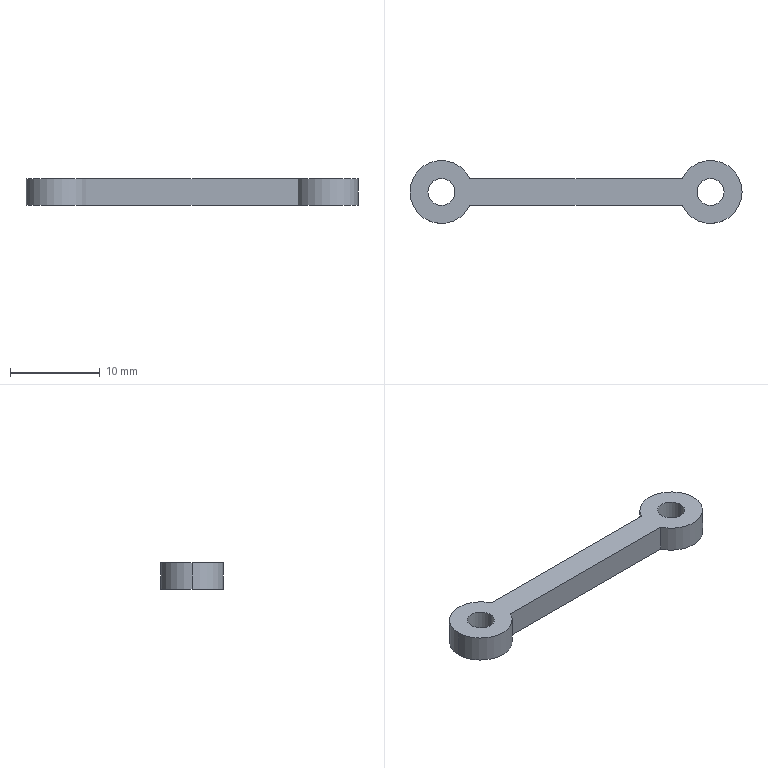Part | STEP file | Small crossbar_1 | 1 solid | 11 faces | box 37 x 7 x 3 mm | volume 397.481 mm3 | cylinder 7 | plane 4 | commonest cylinder face diameters 3 x4 7 x3
STEP:
#1=CARTESIAN_POINT('',(0.,0.,0.));
#2=DIRECTION('',(0.,0.,1.));
#3=DIRECTION('',(1.,0.,0.));
#4=AXIS2_PLACEMENT_3D('',#1,#2,#3);
#5=CARTESIAN_POINT('',(28.5,0.,3.));
#6=VERTEX_POINT('',#5);
#7=CARTESIAN_POINT('',(28.5,0.,0.));
#8=VERTEX_POINT('',#7);
#9=CARTESIAN_POINT('',(28.5,0.,3.));
#10=DIRECTION('',(0.,0.,-1.));
#11=VECTOR('',#10,1.);
#12=LINE('',#9,#11);
#13=CARTESIAN_POINT('',(30.,0.,3.));
#14=DIRECTION('',(0.,0.,-1.));
#15=DIRECTION('',(-1.,0.,0.));
#16=AXIS2_PLACEMENT_3D('',#13,#14,#15);
#17=CYLINDRICAL_SURFACE('',#16,1.5);
#18=CARTESIAN_POINT('',(6.283,0.));
#19=DIRECTION('',(0.,1.));
#20=VECTOR('',#19,1.);
#21=LINE('',#18,#20);
#22=(GEOMETRIC_REPRESENTATION_CONTEXT(2)PARAMETRIC_REPRESENTATION_CONTEXT()REPRESENTATION_CONTEXT('',''));
#23=DEFINITIONAL_REPRESENTATION('',(#21),#22);
#24=PCURVE('',#17,#23);
#25=CARTESIAN_POINT('',(30.,0.,3.));
#26=DIRECTION('',(0.,0.,-1.));
#27=DIRECTION('',(-1.,0.,0.));
#28=AXIS2_PLACEMENT_3D('',#25,#26,#27);
#29=CYLINDRICAL_SURFACE('',#28,1.5);
#30=CARTESIAN_POINT('',(0.,0.));
#31=DIRECTION('',(0.,1.));
#32=VECTOR('',#31,1.);
#33=LINE('',#30,#32);
#34=(GEOMETRIC_REPRESENTATION_CONTEXT(2)PARAMETRIC_REPRESENTATION_CONTEXT()REPRESENTATION_CONTEXT('',''));
#35=DEFINITIONAL_REPRESENTATION('',(#33),#34);
#36=PCURVE('',#29,#35);
#37=SURFACE_CURVE('',#12,(#24,#36),.PCURVE_S1.);
#38=EDGE_CURVE('',#6,#8,#37,.T.);
#39=ORIENTED_EDGE('',*,*,#38,.T.);
#40=CARTESIAN_POINT('',(31.5,0.,0.));
#41=VERTEX_POINT('',#40);
#42=CARTESIAN_POINT('',(30.,0.,0.));
#43=DIRECTION('',(0.,0.,1.));
#44=DIRECTION('',(-1.,0.,0.));
#45=AXIS2_PLACEMENT_3D('',#42,#43,#44);
#46=CIRCLE('',#45,1.5);
#47=CARTESIAN_POINT('',(6.283,3.));
#48=DIRECTION('',(-1.,0.));
#49=VECTOR('',#48,1.);
#50=LINE('',#47,#49);
#51=(GEOMETRIC_REPRESENTATION_CONTEXT(2)PARAMETRIC_REPRESENTATION_CONTEXT()REPRESENTATION_CONTEXT('',''));
#52=DEFINITIONAL_REPRESENTATION('',(#50),#51);
#53=PCURVE('',#17,#52);
#54=CARTESIAN_POINT('',(0.,0.,0.));
#55=DIRECTION('',(0.,0.,1.));
#56=DIRECTION('',(1.,0.,0.));
#57=AXIS2_PLACEMENT_3D('',#54,#55,#56);
#58=PLANE('',#57);
#59=CARTESIAN_POINT('',(30.,0.));
#60=DIRECTION('',(-1.,0.));
#61=AXIS2_PLACEMENT_2D('',#59,#60);
#62=CIRCLE('',#61,1.5);
#63=(GEOMETRIC_REPRESENTATION_CONTEXT(2)PARAMETRIC_REPRESENTATION_CONTEXT()REPRESENTATION_CONTEXT('',''));
#64=DEFINITIONAL_REPRESENTATION('',(#62),#63);
#65=PCURVE('',#58,#64);
#66=SURFACE_CURVE('',#46,(#53,#65),.PCURVE_S1.);
#67=EDGE_CURVE('',#8,#41,#66,.T.);
#68=ORIENTED_EDGE('',*,*,#67,.T.);
#69=CARTESIAN_POINT('',(31.5,0.,3.));
#70=VERTEX_POINT('',#69);
#71=CARTESIAN_POINT('',(31.5,0.,3.));
#72=DIRECTION('',(0.,0.,-1.));
#73=VECTOR('',#72,1.);
#74=LINE('',#71,#73);
#75=CARTESIAN_POINT('',(3.142,0.));
#76=DIRECTION('',(0.,1.));
#77=VECTOR('',#76,1.);
#78=LINE('',#75,#77);
#79=(GEOMETRIC_REPRESENTATION_CONTEXT(2)PARAMETRIC_REPRESENTATION_CONTEXT()REPRESENTATION_CONTEXT('',''));
#80=DEFINITIONAL_REPRESENTATION('',(#78),#79);
#81=PCURVE('',#17,#80);
#82=CARTESIAN_POINT('',(3.142,0.));
#83=DIRECTION('',(0.,1.));
#84=VECTOR('',#83,1.);
#85=LINE('',#82,#84);
#86=(GEOMETRIC_REPRESENTATION_CONTEXT(2)PARAMETRIC_REPRESENTATION_CONTEXT()REPRESENTATION_CONTEXT('',''));
#87=DEFINITIONAL_REPRESENTATION('',(#85),#86);
#88=PCURVE('',#29,#87);
#89=SURFACE_CURVE('',#74,(#81,#88),.PCURVE_S1.);
#90=EDGE_CURVE('',#70,#41,#89,.T.);
#91=ORIENTED_EDGE('',*,*,#90,.F.);
#92=CARTESIAN_POINT('',(30.,0.,3.));
#93=DIRECTION('',(0.,0.,-1.));
#94=DIRECTION('',(-1.,0.,0.));
#95=AXIS2_PLACEMENT_3D('',#92,#93,#94);
#96=CIRCLE('',#95,1.5);
#97=CARTESIAN_POINT('',(0.,0.));
#98=DIRECTION('',(1.,0.));
#99=VECTOR('',#98,1.);
#100=LINE('',#97,#99);
#101=(GEOMETRIC_REPRESENTATION_CONTEXT(2)PARAMETRIC_REPRESENTATION_CONTEXT()REPRESENTATION_CONTEXT('',''));
#102=DEFINITIONAL_REPRESENTATION('',(#100),#101);
#103=PCURVE('',#17,#102);
#104=CARTESIAN_POINT('',(0.,0.,3.));
#105=DIRECTION('',(0.,0.,1.));
#106=DIRECTION('',(1.,0.,0.));
#107=AXIS2_PLACEMENT_3D('',#104,#105,#106);
#108=PLANE('',#107);
#109=CARTESIAN_POINT('',(28.5,0.));
#110=CARTESIAN_POINT('',(28.5,2.598));
#111=CARTESIAN_POINT('',(30.75,1.299));
#112=CARTESIAN_POINT('',(33.,0.));
#113=CARTESIAN_POINT('',(30.75,-1.299));
#114=CARTESIAN_POINT('',(28.5,-2.598));
#115=CARTESIAN_POINT('',(28.5,0.));
#116=(BOUNDED_CURVE()B_SPLINE_CURVE(2,(#109,#110,#111,#112,#113,#114,#115),.UNSPECIFIED.,.T.,.F.)B_SPLINE_CURVE_WITH_KNOTS((1,2,2,2,2,1),(-2.094,0.,2.094,4.189,6.283,8.378),.UNSPECIFIED.)CURVE()GEOMETRIC_REPRESENTATION_ITEM()RATIONAL_B_SPLINE_CURVE((1.,0.5,1.,0.5,1.,0.5,1.))REPRESENTATION_ITEM(''));
#117=(GEOMETRIC_REPRESENTATION_CONTEXT(2)PARAMETRIC_REPRESENTATION_CONTEXT()REPRESENTATION_CONTEXT('',''));
#118=DEFINITIONAL_REPRESENTATION('',(#116),#117);
#119=PCURVE('',#108,#118);
#120=SURFACE_CURVE('',#96,(#103,#119),.PCURVE_S1.);
#121=EDGE_CURVE('',#70,#6,#120,.T.);
#122=ORIENTED_EDGE('',*,*,#121,.T.);
#123=EDGE_LOOP('',(#39,#68,#91,#122));
#124=FACE_BOUND('',#123,.F.);
#125=ADVANCED_FACE('',(#124),#17,.F.);
#126=CARTESIAN_POINT('',(-3.5,0.,3.));
#127=VERTEX_POINT('',#126);
#128=CARTESIAN_POINT('',(3.162,-1.5,3.));
#129=VERTEX_POINT('',#128);
#130=CARTESIAN_POINT('',(0.,0.,3.));
#131=DIRECTION('',(0.,0.,1.));
#132=DIRECTION('',(-1.,0.,0.));
#133=AXIS2_PLACEMENT_3D('',#130,#131,#132);
#134=CIRCLE('',#133,3.5);
#135=CARTESIAN_POINT('',(0.,0.,3.));
#136=DIRECTION('',(0.,0.,-1.));
#137=DIRECTION('',(-1.,0.,0.));
#138=AXIS2_PLACEMENT_3D('',#135,#136,#137);
#139=CYLINDRICAL_SURFACE('',#138,3.5);
#140=CARTESIAN_POINT('',(6.283,0.));
#141=DIRECTION('',(-1.,0.));
#142=VECTOR('',#141,1.);
#143=LINE('',#140,#142);
#144=(GEOMETRIC_REPRESENTATION_CONTEXT(2)PARAMETRIC_REPRESENTATION_CONTEXT()REPRESENTATION_CONTEXT('',''));
#145=DEFINITIONAL_REPRESENTATION('',(#143),#144);
#146=PCURVE('',#139,#145);
#147=CARTESIAN_POINT('',(0.,0.));
#148=DIRECTION('',(-1.,0.));
#149=AXIS2_PLACEMENT_2D('',#147,#148);
#150=CIRCLE('',#149,3.5);
#151=(GEOMETRIC_REPRESENTATION_CONTEXT(2)PARAMETRIC_REPRESENTATION_CONTEXT()REPRESENTATION_CONTEXT('',''));
#152=DEFINITIONAL_REPRESENTATION('',(#150),#151);
#153=PCURVE('',#108,#152);
#154=SURFACE_CURVE('',#134,(#146,#153),.PCURVE_S1.);
#155=EDGE_CURVE('',#127,#129,#154,.T.);
#156=ORIENTED_EDGE('',*,*,#155,.F.);
#157=CARTESIAN_POINT('',(-3.5,0.,0.));
#158=VERTEX_POINT('',#157);
#159=CARTESIAN_POINT('',(-3.5,0.,3.));
#160=DIRECTION('',(0.,0.,-1.));
#161=VECTOR('',#160,1.);
#162=LINE('',#159,#161);
#163=CARTESIAN_POINT('',(6.283,0.));
#164=DIRECTION('',(0.,1.));
#165=VECTOR('',#164,1.);
#166=LINE('',#163,#165);
#167=(GEOMETRIC_REPRESENTATION_CONTEXT(2)PARAMETRIC_REPRESENTATION_CONTEXT()REPRESENTATION_CONTEXT('',''));
#168=DEFINITIONAL_REPRESENTATION('',(#166),#167);
#169=PCURVE('',#139,#168);
#170=CARTESIAN_POINT('',(0.,0.,3.));
#171=DIRECTION('',(0.,0.,-1.));
#172=DIRECTION('',(-1.,0.,0.));
#173=AXIS2_PLACEMENT_3D('',#170,#171,#172);
#174=CYLINDRICAL_SURFACE('',#173,3.5);
#175=CARTESIAN_POINT('',(0.,0.));
#176=DIRECTION('',(0.,1.));
#177=VECTOR('',#176,1.);
#178=LINE('',#175,#177);
#179=(GEOMETRIC_REPRESENTATION_CONTEXT(2)PARAMETRIC_REPRESENTATION_CONTEXT()REPRESENTATION_CONTEXT('',''));
#180=DEFINITIONAL_REPRESENTATION('',(#178),#179);
#181=PCURVE('',#174,#180);
#182=SURFACE_CURVE('',#162,(#169,#181),.PCURVE_S1.);
#183=EDGE_CURVE('',#127,#158,#182,.T.);
#184=ORIENTED_EDGE('',*,*,#183,.T.);
#185=CARTESIAN_POINT('',(3.162,-1.5,0.));
#186=VERTEX_POINT('',#185);
#187=CARTESIAN_POINT('',(0.,0.,0.));
#188=DIRECTION('',(0.,0.,1.));
#189=DIRECTION('',(-1.,0.,0.));
#190=AXIS2_PLACEMENT_3D('',#187,#188,#189);
#191=CIRCLE('',#190,3.5);
#192=CARTESIAN_POINT('',(6.283,3.));
#193=DIRECTION('',(-1.,0.));
#194=VECTOR('',#193,1.);
#195=LINE('',#192,#194);
#196=(GEOMETRIC_REPRESENTATION_CONTEXT(2)PARAMETRIC_REPRESENTATION_CONTEXT()REPRESENTATION_CONTEXT('',''));
#197=DEFINITIONAL_REPRESENTATION('',(#195),#196);
#198=PCURVE('',#139,#197);
#199=CARTESIAN_POINT('',(0.,0.));
#200=DIRECTION('',(-1.,0.));
#201=AXIS2_PLACEMENT_2D('',#199,#200);
#202=CIRCLE('',#201,3.5);
#203=(GEOMETRIC_REPRESENTATION_CONTEXT(2)PARAMETRIC_REPRESENTATION_CONTEXT()REPRESENTATION_CONTEXT('',''));
#204=DEFINITIONAL_REPRESENTATION('',(#202),#203);
#205=PCURVE('',#58,#204);
#206=SURFACE_CURVE('',#191,(#198,#205),.PCURVE_S1.);
#207=EDGE_CURVE('',#158,#186,#206,.T.);
#208=ORIENTED_EDGE('',*,*,#207,.T.);
#209=CARTESIAN_POINT('',(3.162,-1.5,3.));
#210=DIRECTION('',(0.,0.,1.));
#211=VECTOR('',#210,1.);
#212=LINE('',#209,#211);
#213=CARTESIAN_POINT('',(3.585,0.));
#214=DIRECTION('',(0.,-1.));
#215=VECTOR('',#214,1.);
#216=LINE('',#213,#215);
#217=(GEOMETRIC_REPRESENTATION_CONTEXT(2)PARAMETRIC_REPRESENTATION_CONTEXT()REPRESENTATION_CONTEXT('',''));
#218=DEFINITIONAL_REPRESENTATION('',(#216),#217);
#219=PCURVE('',#139,#218);
#220=CARTESIAN_POINT('',(3.162,-1.5,3.));
#221=DIRECTION('',(0.,1.,0.));
#222=DIRECTION('',(0.,0.,1.));
#223=AXIS2_PLACEMENT_3D('',#220,#221,#222);
#224=PLANE('',#223);
#225=CARTESIAN_POINT('',(0.,0.));
#226=DIRECTION('',(1.,0.));
#227=VECTOR('',#226,1.);
#228=LINE('',#225,#227);
#229=(GEOMETRIC_REPRESENTATION_CONTEXT(2)PARAMETRIC_REPRESENTATION_CONTEXT()REPRESENTATION_CONTEXT('',''));
#230=DEFINITIONAL_REPRESENTATION('',(#228),#229);
#231=PCURVE('',#224,#230);
#232=SURFACE_CURVE('',#212,(#219,#231),.PCURVE_S1.);
#233=EDGE_CURVE('',#186,#129,#232,.T.);
#234=ORIENTED_EDGE('',*,*,#233,.T.);
#235=EDGE_LOOP('',(#156,#184,#208,#234));
#236=FACE_BOUND('',#235,.T.);
#237=ADVANCED_FACE('',(#236),#139,.T.);
#238=CARTESIAN_POINT('',(-1.5,0.,3.));
#239=VERTEX_POINT('',#238);
#240=CARTESIAN_POINT('',(-1.5,0.,0.));
#241=VERTEX_POINT('',#240);
#242=CARTESIAN_POINT('',(-1.5,0.,3.));
#243=DIRECTION('',(0.,0.,-1.));
#244=VECTOR('',#243,1.);
#245=LINE('',#242,#244);
#246=CARTESIAN_POINT('',(0.,0.,3.));
#247=DIRECTION('',(0.,0.,-1.));
#248=DIRECTION('',(-1.,0.,0.));
#249=AXIS2_PLACEMENT_3D('',#246,#247,#248);
#250=CYLINDRICAL_SURFACE('',#249,1.5);
#251=CARTESIAN_POINT('',(6.283,0.));
#252=DIRECTION('',(0.,1.));
#253=VECTOR('',#252,1.);
#254=LINE('',#251,#253);
#255=(GEOMETRIC_REPRESENTATION_CONTEXT(2)PARAMETRIC_REPRESENTATION_CONTEXT()REPRESENTATION_CONTEXT('',''));
#256=DEFINITIONAL_REPRESENTATION('',(#254),#255);
#257=PCURVE('',#250,#256);
#258=CARTESIAN_POINT('',(0.,0.,3.));
#259=DIRECTION('',(0.,0.,-1.));
#260=DIRECTION('',(-1.,0.,0.));
#261=AXIS2_PLACEMENT_3D('',#258,#259,#260);
#262=CYLINDRICAL_SURFACE('',#261,1.5);
#263=CARTESIAN_POINT('',(0.,0.));
#264=DIRECTION('',(0.,1.));
#265=VECTOR('',#264,1.);
#266=LINE('',#263,#265);
#267=(GEOMETRIC_REPRESENTATION_CONTEXT(2)PARAMETRIC_REPRESENTATION_CONTEXT()REPRESENTATION_CONTEXT('',''));
#268=DEFINITIONAL_REPRESENTATION('',(#266),#267);
#269=PCURVE('',#262,#268);
#270=SURFACE_CURVE('',#245,(#257,#269),.PCURVE_S1.);
#271=EDGE_CURVE('',#239,#241,#270,.T.);
#272=ORIENTED_EDGE('',*,*,#271,.T.);
#273=CARTESIAN_POINT('',(1.5,0.,0.));
#274=VERTEX_POINT('',#273);
#275=CARTESIAN_POINT('',(0.,0.,0.));
#276=DIRECTION('',(0.,0.,1.));
#277=DIRECTION('',(-1.,0.,0.));
#278=AXIS2_PLACEMENT_3D('',#275,#276,#277);
#279=CIRCLE('',#278,1.5);
#280=CARTESIAN_POINT('',(6.283,3.));
#281=DIRECTION('',(-1.,0.));
#282=VECTOR('',#281,1.);
#283=LINE('',#280,#282);
#284=(GEOMETRIC_REPRESENTATION_CONTEXT(2)PARAMETRIC_REPRESENTATION_CONTEXT()REPRESENTATION_CONTEXT('',''));
#285=DEFINITIONAL_REPRESENTATION('',(#283),#284);
#286=PCURVE('',#250,#285);
#287=CARTESIAN_POINT('',(0.,0.));
#288=DIRECTION('',(-1.,0.));
#289=AXIS2_PLACEMENT_2D('',#287,#288);
#290=CIRCLE('',#289,1.5);
#291=(GEOMETRIC_REPRESENTATION_CONTEXT(2)PARAMETRIC_REPRESENTATION_CONTEXT()REPRESENTATION_CONTEXT('',''));
#292=DEFINITIONAL_REPRESENTATION('',(#290),#291);
#293=PCURVE('',#58,#292);
#294=SURFACE_CURVE('',#279,(#286,#293),.PCURVE_S1.);
#295=EDGE_CURVE('',#241,#274,#294,.T.);
#296=ORIENTED_EDGE('',*,*,#295,.T.);
#297=CARTESIAN_POINT('',(1.5,0.,3.));
#298=VERTEX_POINT('',#297);
#299=CARTESIAN_POINT('',(1.5,0.,3.));
#300=DIRECTION('',(0.,0.,-1.));
#301=VECTOR('',#300,1.);
#302=LINE('',#299,#301);
#303=CARTESIAN_POINT('',(3.142,0.));
#304=DIRECTION('',(0.,1.));
#305=VECTOR('',#304,1.);
#306=LINE('',#303,#305);
#307=(GEOMETRIC_REPRESENTATION_CONTEXT(2)PARAMETRIC_REPRESENTATION_CONTEXT()REPRESENTATION_CONTEXT('',''));
#308=DEFINITIONAL_REPRESENTATION('',(#306),#307);
#309=PCURVE('',#250,#308);
#310=CARTESIAN_POINT('',(3.142,0.));
#311=DIRECTION('',(0.,1.));
#312=VECTOR('',#311,1.);
#313=LINE('',#310,#312);
#314=(GEOMETRIC_REPRESENTATION_CONTEXT(2)PARAMETRIC_REPRESENTATION_CONTEXT()REPRESENTATION_CONTEXT('',''));
#315=DEFINITIONAL_REPRESENTATION('',(#313),#314);
#316=PCURVE('',#262,#315);
#317=SURFACE_CURVE('',#302,(#309,#316),.PCURVE_S1.);
#318=EDGE_CURVE('',#298,#274,#317,.T.);
#319=ORIENTED_EDGE('',*,*,#318,.F.);
#320=CARTESIAN_POINT('',(0.,0.,3.));
#321=DIRECTION('',(0.,0.,-1.));
#322=DIRECTION('',(-1.,0.,0.));
#323=AXIS2_PLACEMENT_3D('',#320,#321,#322);
#324=CIRCLE('',#323,1.5);
#325=CARTESIAN_POINT('',(0.,0.));
#326=DIRECTION('',(1.,0.));
#327=VECTOR('',#326,1.);
#328=LINE('',#325,#327);
#329=(GEOMETRIC_REPRESENTATION_CONTEXT(2)PARAMETRIC_REPRESENTATION_CONTEXT()REPRESENTATION_CONTEXT('',''));
#330=DEFINITIONAL_REPRESENTATION('',(#328),#329);
#331=PCURVE('',#250,#330);
#332=CARTESIAN_POINT('',(-1.5,0.));
#333=CARTESIAN_POINT('',(-1.5,2.598));
#334=CARTESIAN_POINT('',(0.75,1.299));
#335=CARTESIAN_POINT('',(3.,0.));
#336=CARTESIAN_POINT('',(0.75,-1.299));
#337=CARTESIAN_POINT('',(-1.5,-2.598));
#338=CARTESIAN_POINT('',(-1.5,0.));
#339=(BOUNDED_CURVE()B_SPLINE_CURVE(2,(#332,#333,#334,#335,#336,#337,#338),.UNSPECIFIED.,.T.,.F.)B_SPLINE_CURVE_WITH_KNOTS((1,2,2,2,2,1),(-2.094,0.,2.094,4.189,6.283,8.378),.UNSPECIFIED.)CURVE()GEOMETRIC_REPRESENTATION_ITEM()RATIONAL_B_SPLINE_CURVE((1.,0.5,1.,0.5,1.,0.5,1.))REPRESENTATION_ITEM(''));
#340=(GEOMETRIC_REPRESENTATION_CONTEXT(2)PARAMETRIC_REPRESENTATION_CONTEXT()REPRESENTATION_CONTEXT('',''));
#341=DEFINITIONAL_REPRESENTATION('',(#339),#340);
#342=PCURVE('',#108,#341);
#343=SURFACE_CURVE('',#324,(#331,#342),.PCURVE_S1.);
#344=EDGE_CURVE('',#298,#239,#343,.T.);
#345=ORIENTED_EDGE('',*,*,#344,.T.);
#346=EDGE_LOOP('',(#272,#296,#319,#345));
#347=FACE_BOUND('',#346,.F.);
#348=ADVANCED_FACE('',(#347),#250,.F.);
#349=CARTESIAN_POINT('',(30.,0.,3.));
#350=DIRECTION('',(0.,0.,-1.));
#351=DIRECTION('',(-1.,0.,0.));
#352=AXIS2_PLACEMENT_3D('',#349,#350,#351);
#353=CIRCLE('',#352,1.5);
#354=CARTESIAN_POINT('',(28.5,0.));
#355=CARTESIAN_POINT('',(28.5,2.598));
#356=CARTESIAN_POINT('',(30.75,1.299));
#357=CARTESIAN_POINT('',(33.,0.));
#358=CARTESIAN_POINT('',(30.75,-1.299));
#359=CARTESIAN_POINT('',(28.5,-2.598));
#360=CARTESIAN_POINT('',(28.5,0.));
#361=(BOUNDED_CURVE()B_SPLINE_CURVE(2,(#354,#355,#356,#357,#358,#359,#360),.UNSPECIFIED.,.T.,.F.)B_SPLINE_CURVE_WITH_KNOTS((1,2,2,2,2,1),(-2.094,0.,2.094,4.189,6.283,8.378),.UNSPECIFIED.)CURVE()GEOMETRIC_REPRESENTATION_ITEM()RATIONAL_B_SPLINE_CURVE((1.,0.5,1.,0.5,1.,0.5,1.))REPRESENTATION_ITEM(''));
#362=(GEOMETRIC_REPRESENTATION_CONTEXT(2)PARAMETRIC_REPRESENTATION_CONTEXT()REPRESENTATION_CONTEXT('',''));
#363=DEFINITIONAL_REPRESENTATION('',(#361),#362);
#364=PCURVE('',#108,#363);
#365=CARTESIAN_POINT('',(0.,0.));
#366=DIRECTION('',(1.,0.));
#367=VECTOR('',#366,1.);
#368=LINE('',#365,#367);
#369=(GEOMETRIC_REPRESENTATION_CONTEXT(2)PARAMETRIC_REPRESENTATION_CONTEXT()REPRESENTATION_CONTEXT('',''));
#370=DEFINITIONAL_REPRESENTATION('',(#368),#369);
#371=PCURVE('',#29,#370);
#372=SURFACE_CURVE('',#353,(#364,#371),.PCURVE_S1.);
#373=EDGE_CURVE('',#6,#70,#372,.T.);
#374=ORIENTED_EDGE('',*,*,#373,.T.);
#375=ORIENTED_EDGE('',*,*,#121,.T.);
#376=EDGE_LOOP('',(#374,#375));
#377=FACE_BOUND('',#376,.T.);
#378=CARTESIAN_POINT('',(26.838,-1.5,3.));
#379=VERTEX_POINT('',#378);
#380=CARTESIAN_POINT('',(26.838,1.5,3.));
#381=VERTEX_POINT('',#380);
#382=CARTESIAN_POINT('',(30.,0.,3.));
#383=DIRECTION('',(0.,0.,1.));
#384=DIRECTION('',(-1.,0.,0.));
#385=AXIS2_PLACEMENT_3D('',#382,#383,#384);
#386=CIRCLE('',#385,3.5);
#387=CARTESIAN_POINT('',(30.,0.));
#388=DIRECTION('',(-1.,0.));
#389=AXIS2_PLACEMENT_2D('',#387,#388);
#390=CIRCLE('',#389,3.5);
#391=(GEOMETRIC_REPRESENTATION_CONTEXT(2)PARAMETRIC_REPRESENTATION_CONTEXT()REPRESENTATION_CONTEXT('',''));
#392=DEFINITIONAL_REPRESENTATION('',(#390),#391);
#393=PCURVE('',#108,#392);
#394=CARTESIAN_POINT('',(30.,0.,3.));
#395=DIRECTION('',(0.,0.,-1.));
#396=DIRECTION('',(-1.,0.,0.));
#397=AXIS2_PLACEMENT_3D('',#394,#395,#396);
#398=CYLINDRICAL_SURFACE('',#397,3.5);
#399=CARTESIAN_POINT('',(6.283,0.));
#400=DIRECTION('',(-1.,0.));
#401=VECTOR('',#400,1.);
#402=LINE('',#399,#401);
#403=(GEOMETRIC_REPRESENTATION_CONTEXT(2)PARAMETRIC_REPRESENTATION_CONTEXT()REPRESENTATION_CONTEXT('',''));
#404=DEFINITIONAL_REPRESENTATION('',(#402),#403);
#405=PCURVE('',#398,#404);
#406=SURFACE_CURVE('',#386,(#393,#405),.PCURVE_S1.);
#407=EDGE_CURVE('',#379,#381,#406,.T.);
#408=ORIENTED_EDGE('',*,*,#407,.T.);
#409=CARTESIAN_POINT('',(3.162,1.5,3.));
#410=VERTEX_POINT('',#409);
#411=CARTESIAN_POINT('',(0.,1.5,3.));
#412=DIRECTION('',(-1.,0.,0.));
#413=VECTOR('',#412,1.);
#414=LINE('',#411,#413);
#415=CARTESIAN_POINT('',(0.,1.5));
#416=DIRECTION('',(-1.,0.));
#417=VECTOR('',#416,1.);
#418=LINE('',#415,#417);
#419=(GEOMETRIC_REPRESENTATION_CONTEXT(2)PARAMETRIC_REPRESENTATION_CONTEXT()REPRESENTATION_CONTEXT('',''));
#420=DEFINITIONAL_REPRESENTATION('',(#418),#419);
#421=PCURVE('',#108,#420);
#422=CARTESIAN_POINT('',(3.162,1.5,3.));
#423=DIRECTION('',(0.,-1.,0.));
#424=DIRECTION('',(0.,0.,-1.));
#425=AXIS2_PLACEMENT_3D('',#422,#423,#424);
#426=PLANE('',#425);
#427=CARTESIAN_POINT('',(0.,-3.162));
#428=DIRECTION('',(0.,-1.));
#429=VECTOR('',#428,1.);
#430=LINE('',#427,#429);
#431=(GEOMETRIC_REPRESENTATION_CONTEXT(2)PARAMETRIC_REPRESENTATION_CONTEXT()REPRESENTATION_CONTEXT('',''));
#432=DEFINITIONAL_REPRESENTATION('',(#430),#431);
#433=PCURVE('',#426,#432);
#434=SURFACE_CURVE('',#414,(#421,#433),.PCURVE_S1.);
#435=EDGE_CURVE('',#381,#410,#434,.T.);
#436=ORIENTED_EDGE('',*,*,#435,.T.);
#437=CARTESIAN_POINT('',(0.,0.,3.));
#438=DIRECTION('',(0.,0.,1.));
#439=DIRECTION('',(-1.,0.,0.));
#440=AXIS2_PLACEMENT_3D('',#437,#438,#439);
#441=CIRCLE('',#440,3.5);
#442=CARTESIAN_POINT('',(0.,0.));
#443=DIRECTION('',(-1.,0.));
#444=AXIS2_PLACEMENT_2D('',#442,#443);
#445=CIRCLE('',#444,3.5);
#446=(GEOMETRIC_REPRESENTATION_CONTEXT(2)PARAMETRIC_REPRESENTATION_CONTEXT()REPRESENTATION_CONTEXT('',''));
#447=DEFINITIONAL_REPRESENTATION('',(#445),#446);
#448=PCURVE('',#108,#447);
#449=CARTESIAN_POINT('',(6.283,0.));
#450=DIRECTION('',(-1.,0.));
#451=VECTOR('',#450,1.);
#452=LINE('',#449,#451);
#453=(GEOMETRIC_REPRESENTATION_CONTEXT(2)PARAMETRIC_REPRESENTATION_CONTEXT()REPRESENTATION_CONTEXT('',''));
#454=DEFINITIONAL_REPRESENTATION('',(#452),#453);
#455=PCURVE('',#174,#454);
#456=SURFACE_CURVE('',#441,(#448,#455),.PCURVE_S1.);
#457=EDGE_CURVE('',#410,#127,#456,.T.);
#458=ORIENTED_EDGE('',*,*,#457,.T.);
#459=ORIENTED_EDGE('',*,*,#155,.T.);
#460=CARTESIAN_POINT('',(0.,-1.5,3.));
#461=DIRECTION('',(1.,0.,0.));
#462=VECTOR('',#461,1.);
#463=LINE('',#460,#462);
#464=CARTESIAN_POINT('',(0.,-1.5));
#465=DIRECTION('',(1.,0.));
#466=VECTOR('',#465,1.);
#467=LINE('',#464,#466);
#468=(GEOMETRIC_REPRESENTATION_CONTEXT(2)PARAMETRIC_REPRESENTATION_CONTEXT()REPRESENTATION_CONTEXT('',''));
#469=DEFINITIONAL_REPRESENTATION('',(#467),#468);
#470=PCURVE('',#108,#469);
#471=CARTESIAN_POINT('',(0.,-3.162));
#472=DIRECTION('',(0.,1.));
#473=VECTOR('',#472,1.);
#474=LINE('',#471,#473);
#475=(GEOMETRIC_REPRESENTATION_CONTEXT(2)PARAMETRIC_REPRESENTATION_CONTEXT()REPRESENTATION_CONTEXT('',''));
#476=DEFINITIONAL_REPRESENTATION('',(#474),#475);
#477=PCURVE('',#224,#476);
#478=SURFACE_CURVE('',#463,(#470,#477),.PCURVE_S1.);
#479=EDGE_CURVE('',#129,#379,#478,.T.);
#480=ORIENTED_EDGE('',*,*,#479,.T.);
#481=EDGE_LOOP('',(#408,#436,#458,#459,#480));
#482=FACE_BOUND('',#481,.T.);
#483=CARTESIAN_POINT('',(0.,0.,3.));
#484=DIRECTION('',(0.,0.,-1.));
#485=DIRECTION('',(-1.,0.,0.));
#486=AXIS2_PLACEMENT_3D('',#483,#484,#485);
#487=CIRCLE('',#486,1.5);
#488=CARTESIAN_POINT('',(-1.5,0.));
#489=CARTESIAN_POINT('',(-1.5,2.598));
#490=CARTESIAN_POINT('',(0.75,1.299));
#491=CARTESIAN_POINT('',(3.,0.));
#492=CARTESIAN_POINT('',(0.75,-1.299));
#493=CARTESIAN_POINT('',(-1.5,-2.598));
#494=CARTESIAN_POINT('',(-1.5,0.));
#495=(BOUNDED_CURVE()B_SPLINE_CURVE(2,(#488,#489,#490,#491,#492,#493,#494),.UNSPECIFIED.,.T.,.F.)B_SPLINE_CURVE_WITH_KNOTS((1,2,2,2,2,1),(-2.094,0.,2.094,4.189,6.283,8.378),.UNSPECIFIED.)CURVE()GEOMETRIC_REPRESENTATION_ITEM()RATIONAL_B_SPLINE_CURVE((1.,0.5,1.,0.5,1.,0.5,1.))REPRESENTATION_ITEM(''));
#496=(GEOMETRIC_REPRESENTATION_CONTEXT(2)PARAMETRIC_REPRESENTATION_CONTEXT()REPRESENTATION_CONTEXT('',''));
#497=DEFINITIONAL_REPRESENTATION('',(#495),#496);
#498=PCURVE('',#108,#497);
#499=CARTESIAN_POINT('',(0.,0.));
#500=DIRECTION('',(1.,0.));
#501=VECTOR('',#500,1.);
#502=LINE('',#499,#501);
#503=(GEOMETRIC_REPRESENTATION_CONTEXT(2)PARAMETRIC_REPRESENTATION_CONTEXT()REPRESENTATION_CONTEXT('',''));
#504=DEFINITIONAL_REPRESENTATION('',(#502),#503);
#505=PCURVE('',#262,#504);
#506=SURFACE_CURVE('',#487,(#498,#505),.PCURVE_S1.);
#507=EDGE_CURVE('',#239,#298,#506,.T.);
#508=ORIENTED_EDGE('',*,*,#507,.T.);
#509=ORIENTED_EDGE('',*,*,#344,.T.);
#510=EDGE_LOOP('',(#508,#509));
#511=FACE_BOUND('',#510,.T.);
#512=ADVANCED_FACE('',(#377,#482,#511),#108,.T.);
#513=CARTESIAN_POINT('',(30.,0.,0.));
#514=DIRECTION('',(0.,0.,1.));
#515=DIRECTION('',(-1.,0.,0.));
#516=AXIS2_PLACEMENT_3D('',#513,#514,#515);
#517=CIRCLE('',#516,1.5);
#518=CARTESIAN_POINT('',(6.283,3.));
#519=DIRECTION('',(-1.,0.));
#520=VECTOR('',#519,1.);
#521=LINE('',#518,#520);
#522=(GEOMETRIC_REPRESENTATION_CONTEXT(2)PARAMETRIC_REPRESENTATION_CONTEXT()REPRESENTATION_CONTEXT('',''));
#523=DEFINITIONAL_REPRESENTATION('',(#521),#522);
#524=PCURVE('',#29,#523);
#525=CARTESIAN_POINT('',(30.,0.));
#526=DIRECTION('',(-1.,0.));
#527=AXIS2_PLACEMENT_2D('',#525,#526);
#528=CIRCLE('',#527,1.5);
#529=(GEOMETRIC_REPRESENTATION_CONTEXT(2)PARAMETRIC_REPRESENTATION_CONTEXT()REPRESENTATION_CONTEXT('',''));
#530=DEFINITIONAL_REPRESENTATION('',(#528),#529);
#531=PCURVE('',#58,#530);
#532=SURFACE_CURVE('',#517,(#524,#531),.PCURVE_S1.);
#533=EDGE_CURVE('',#41,#8,#532,.T.);
#534=ORIENTED_EDGE('',*,*,#533,.T.);
#535=ORIENTED_EDGE('',*,*,#38,.F.);
#536=ORIENTED_EDGE('',*,*,#373,.T.);
#537=ORIENTED_EDGE('',*,*,#90,.T.);
#538=EDGE_LOOP('',(#534,#535,#536,#537));
#539=FACE_BOUND('',#538,.F.);
#540=ADVANCED_FACE('',(#539),#29,.F.);
#541=CARTESIAN_POINT('',(3.162,1.5,0.));
#542=VERTEX_POINT('',#541);
#543=CARTESIAN_POINT('',(3.162,1.5,3.));
#544=DIRECTION('',(0.,0.,-1.));
#545=VECTOR('',#544,1.);
#546=LINE('',#543,#545);
#547=CARTESIAN_POINT('',(0.,0.));
#548=DIRECTION('',(1.,0.));
#549=VECTOR('',#548,1.);
#550=LINE('',#547,#549);
#551=(GEOMETRIC_REPRESENTATION_CONTEXT(2)PARAMETRIC_REPRESENTATION_CONTEXT()REPRESENTATION_CONTEXT('',''));
#552=DEFINITIONAL_REPRESENTATION('',(#550),#551);
#553=PCURVE('',#426,#552);
#554=CARTESIAN_POINT('',(2.699,0.));
#555=DIRECTION('',(0.,1.));
#556=VECTOR('',#555,1.);
#557=LINE('',#554,#556);
#558=(GEOMETRIC_REPRESENTATION_CONTEXT(2)PARAMETRIC_REPRESENTATION_CONTEXT()REPRESENTATION_CONTEXT('',''));
#559=DEFINITIONAL_REPRESENTATION('',(#557),#558);
#560=PCURVE('',#174,#559);
#561=SURFACE_CURVE('',#546,(#553,#560),.PCURVE_S1.);
#562=EDGE_CURVE('',#410,#542,#561,.T.);
#563=ORIENTED_EDGE('',*,*,#562,.F.);
#564=ORIENTED_EDGE('',*,*,#435,.F.);
#565=CARTESIAN_POINT('',(26.838,1.5,0.));
#566=VERTEX_POINT('',#565);
#567=CARTESIAN_POINT('',(26.838,1.5,3.));
#568=DIRECTION('',(0.,0.,1.));
#569=VECTOR('',#568,1.);
#570=LINE('',#567,#569);
#571=CARTESIAN_POINT('',(0.,23.675));
#572=DIRECTION('',(-1.,0.));
#573=VECTOR('',#572,1.);
#574=LINE('',#571,#573);
#575=(GEOMETRIC_REPRESENTATION_CONTEXT(2)PARAMETRIC_REPRESENTATION_CONTEXT()REPRESENTATION_CONTEXT('',''));
#576=DEFINITIONAL_REPRESENTATION('',(#574),#575);
#577=PCURVE('',#426,#576);
#578=CARTESIAN_POINT('',(0.4429,0.));
#579=DIRECTION('',(0.,-1.));
#580=VECTOR('',#579,1.);
#581=LINE('',#578,#580);
#582=(GEOMETRIC_REPRESENTATION_CONTEXT(2)PARAMETRIC_REPRESENTATION_CONTEXT()REPRESENTATION_CONTEXT('',''));
#583=DEFINITIONAL_REPRESENTATION('',(#581),#582);
#584=PCURVE('',#398,#583);
#585=SURFACE_CURVE('',#570,(#577,#584),.PCURVE_S1.);
#586=EDGE_CURVE('',#566,#381,#585,.T.);
#587=ORIENTED_EDGE('',*,*,#586,.F.);
#588=CARTESIAN_POINT('',(3.162,1.5,0.));
#589=DIRECTION('',(1.,0.,0.));
#590=VECTOR('',#589,1.);
#591=LINE('',#588,#590);
#592=CARTESIAN_POINT('',(3.,0.));
#593=DIRECTION('',(0.,1.));
#594=VECTOR('',#593,1.);
#595=LINE('',#592,#594);
#596=(GEOMETRIC_REPRESENTATION_CONTEXT(2)PARAMETRIC_REPRESENTATION_CONTEXT()REPRESENTATION_CONTEXT('',''));
#597=DEFINITIONAL_REPRESENTATION('',(#595),#596);
#598=PCURVE('',#426,#597);
#599=CARTESIAN_POINT('',(3.162,1.5));
#600=DIRECTION('',(1.,0.));
#601=VECTOR('',#600,1.);
#602=LINE('',#599,#601);
#603=(GEOMETRIC_REPRESENTATION_CONTEXT(2)PARAMETRIC_REPRESENTATION_CONTEXT()REPRESENTATION_CONTEXT('',''));
#604=DEFINITIONAL_REPRESENTATION('',(#602),#603);
#605=PCURVE('',#58,#604);
#606=SURFACE_CURVE('',#591,(#598,#605),.PCURVE_S1.);
#607=EDGE_CURVE('',#542,#566,#606,.T.);
#608=ORIENTED_EDGE('',*,*,#607,.F.);
#609=EDGE_LOOP('',(#563,#564,#587,#608));
#610=FACE_BOUND('',#609,.T.);
#611=ADVANCED_FACE('',(#610),#426,.F.);
#612=ORIENTED_EDGE('',*,*,#407,.F.);
#613=CARTESIAN_POINT('',(26.838,-1.5,0.));
#614=VERTEX_POINT('',#613);
#615=CARTESIAN_POINT('',(26.838,-1.5,3.));
#616=DIRECTION('',(0.,0.,-1.));
#617=VECTOR('',#616,1.);
#618=LINE('',#615,#617);
#619=CARTESIAN_POINT('',(5.84,0.));
#620=DIRECTION('',(0.,1.));
#621=VECTOR('',#620,1.);
#622=LINE('',#619,#621);
#623=(GEOMETRIC_REPRESENTATION_CONTEXT(2)PARAMETRIC_REPRESENTATION_CONTEXT()REPRESENTATION_CONTEXT('',''));
#624=DEFINITIONAL_REPRESENTATION('',(#622),#623);
#625=PCURVE('',#398,#624);
#626=CARTESIAN_POINT('',(0.,23.675));
#627=DIRECTION('',(-1.,0.));
#628=VECTOR('',#627,1.);
#629=LINE('',#626,#628);
#630=(GEOMETRIC_REPRESENTATION_CONTEXT(2)PARAMETRIC_REPRESENTATION_CONTEXT()REPRESENTATION_CONTEXT('',''));
#631=DEFINITIONAL_REPRESENTATION('',(#629),#630);
#632=PCURVE('',#224,#631);
#633=SURFACE_CURVE('',#618,(#625,#632),.PCURVE_S1.);
#634=EDGE_CURVE('',#379,#614,#633,.T.);
#635=ORIENTED_EDGE('',*,*,#634,.T.);
#636=CARTESIAN_POINT('',(30.,0.,0.));
#637=DIRECTION('',(0.,0.,1.));
#638=DIRECTION('',(-1.,0.,0.));
#639=AXIS2_PLACEMENT_3D('',#636,#637,#638);
#640=CIRCLE('',#639,3.5);
#641=CARTESIAN_POINT('',(6.283,3.));
#642=DIRECTION('',(-1.,0.));
#643=VECTOR('',#642,1.);
#644=LINE('',#641,#643);
#645=(GEOMETRIC_REPRESENTATION_CONTEXT(2)PARAMETRIC_REPRESENTATION_CONTEXT()REPRESENTATION_CONTEXT('',''));
#646=DEFINITIONAL_REPRESENTATION('',(#644),#645);
#647=PCURVE('',#398,#646);
#648=CARTESIAN_POINT('',(30.,0.));
#649=DIRECTION('',(-1.,0.));
#650=AXIS2_PLACEMENT_2D('',#648,#649);
#651=CIRCLE('',#650,3.5);
#652=(GEOMETRIC_REPRESENTATION_CONTEXT(2)PARAMETRIC_REPRESENTATION_CONTEXT()REPRESENTATION_CONTEXT('',''));
#653=DEFINITIONAL_REPRESENTATION('',(#651),#652);
#654=PCURVE('',#58,#653);
#655=SURFACE_CURVE('',#640,(#647,#654),.PCURVE_S1.);
#656=EDGE_CURVE('',#614,#566,#655,.T.);
#657=ORIENTED_EDGE('',*,*,#656,.T.);
#658=ORIENTED_EDGE('',*,*,#586,.T.);
#659=EDGE_LOOP('',(#612,#635,#657,#658));
#660=FACE_BOUND('',#659,.T.);
#661=ADVANCED_FACE('',(#660),#398,.T.);
#662=ORIENTED_EDGE('',*,*,#634,.F.);
#663=ORIENTED_EDGE('',*,*,#479,.F.);
#664=ORIENTED_EDGE('',*,*,#233,.F.);
#665=CARTESIAN_POINT('',(3.162,-1.5,0.));
#666=DIRECTION('',(-1.,0.,0.));
#667=VECTOR('',#666,1.);
#668=LINE('',#665,#667);
#669=CARTESIAN_POINT('',(-3.,0.));
#670=DIRECTION('',(0.,-1.));
#671=VECTOR('',#670,1.);
#672=LINE('',#669,#671);
#673=(GEOMETRIC_REPRESENTATION_CONTEXT(2)PARAMETRIC_REPRESENTATION_CONTEXT()REPRESENTATION_CONTEXT('',''));
#674=DEFINITIONAL_REPRESENTATION('',(#672),#673);
#675=PCURVE('',#224,#674);
#676=CARTESIAN_POINT('',(3.162,-1.5));
#677=DIRECTION('',(-1.,0.));
#678=VECTOR('',#677,1.);
#679=LINE('',#676,#678);
#680=(GEOMETRIC_REPRESENTATION_CONTEXT(2)PARAMETRIC_REPRESENTATION_CONTEXT()REPRESENTATION_CONTEXT('',''));
#681=DEFINITIONAL_REPRESENTATION('',(#679),#680);
#682=PCURVE('',#58,#681);
#683=SURFACE_CURVE('',#668,(#675,#682),.PCURVE_S1.);
#684=EDGE_CURVE('',#614,#186,#683,.T.);
#685=ORIENTED_EDGE('',*,*,#684,.F.);
#686=EDGE_LOOP('',(#662,#663,#664,#685));
#687=FACE_BOUND('',#686,.T.);
#688=ADVANCED_FACE('',(#687),#224,.F.);
#689=ORIENTED_EDGE('',*,*,#183,.F.);
#690=ORIENTED_EDGE('',*,*,#457,.F.);
#691=ORIENTED_EDGE('',*,*,#562,.T.);
#692=CARTESIAN_POINT('',(0.,0.,0.));
#693=DIRECTION('',(0.,0.,1.));
#694=DIRECTION('',(-1.,0.,0.));
#695=AXIS2_PLACEMENT_3D('',#692,#693,#694);
#696=CIRCLE('',#695,3.5);
#697=CARTESIAN_POINT('',(6.283,3.));
#698=DIRECTION('',(-1.,0.));
#699=VECTOR('',#698,1.);
#700=LINE('',#697,#699);
#701=(GEOMETRIC_REPRESENTATION_CONTEXT(2)PARAMETRIC_REPRESENTATION_CONTEXT()REPRESENTATION_CONTEXT('',''));
#702=DEFINITIONAL_REPRESENTATION('',(#700),#701);
#703=PCURVE('',#174,#702);
#704=CARTESIAN_POINT('',(0.,0.));
#705=DIRECTION('',(-1.,0.));
#706=AXIS2_PLACEMENT_2D('',#704,#705);
#707=CIRCLE('',#706,3.5);
#708=(GEOMETRIC_REPRESENTATION_CONTEXT(2)PARAMETRIC_REPRESENTATION_CONTEXT()REPRESENTATION_CONTEXT('',''));
#709=DEFINITIONAL_REPRESENTATION('',(#707),#708);
#710=PCURVE('',#58,#709);
#711=SURFACE_CURVE('',#696,(#703,#710),.PCURVE_S1.);
#712=EDGE_CURVE('',#542,#158,#711,.T.);
#713=ORIENTED_EDGE('',*,*,#712,.T.);
#714=EDGE_LOOP('',(#689,#690,#691,#713));
#715=FACE_BOUND('',#714,.T.);
#716=ADVANCED_FACE('',(#715),#174,.T.);
#717=CARTESIAN_POINT('',(0.,0.,0.));
#718=DIRECTION('',(0.,0.,1.));
#719=DIRECTION('',(-1.,0.,0.));
#720=AXIS2_PLACEMENT_3D('',#717,#718,#719);
#721=CIRCLE('',#720,1.5);
#722=CARTESIAN_POINT('',(6.283,3.));
#723=DIRECTION('',(-1.,0.));
#724=VECTOR('',#723,1.);
#725=LINE('',#722,#724);
#726=(GEOMETRIC_REPRESENTATION_CONTEXT(2)PARAMETRIC_REPRESENTATION_CONTEXT()REPRESENTATION_CONTEXT('',''));
#727=DEFINITIONAL_REPRESENTATION('',(#725),#726);
#728=PCURVE('',#262,#727);
#729=CARTESIAN_POINT('',(0.,0.));
#730=DIRECTION('',(-1.,0.));
#731=AXIS2_PLACEMENT_2D('',#729,#730);
#732=CIRCLE('',#731,1.5);
#733=(GEOMETRIC_REPRESENTATION_CONTEXT(2)PARAMETRIC_REPRESENTATION_CONTEXT()REPRESENTATION_CONTEXT('',''));
#734=DEFINITIONAL_REPRESENTATION('',(#732),#733);
#735=PCURVE('',#58,#734);
#736=SURFACE_CURVE('',#721,(#728,#735),.PCURVE_S1.);
#737=EDGE_CURVE('',#274,#241,#736,.T.);
#738=ORIENTED_EDGE('',*,*,#737,.T.);
#739=ORIENTED_EDGE('',*,*,#271,.F.);
#740=ORIENTED_EDGE('',*,*,#507,.T.);
#741=ORIENTED_EDGE('',*,*,#318,.T.);
#742=EDGE_LOOP('',(#738,#739,#740,#741));
#743=FACE_BOUND('',#742,.F.);
#744=ADVANCED_FACE('',(#743),#262,.F.);
#745=ORIENTED_EDGE('',*,*,#67,.T.);
#746=ORIENTED_EDGE('',*,*,#533,.T.);
#747=EDGE_LOOP('',(#745,#746));
#748=FACE_BOUND('',#747,.T.);
#749=ORIENTED_EDGE('',*,*,#607,.T.);
#750=ORIENTED_EDGE('',*,*,#656,.F.);
#751=ORIENTED_EDGE('',*,*,#684,.T.);
#752=ORIENTED_EDGE('',*,*,#207,.F.);
#753=ORIENTED_EDGE('',*,*,#712,.F.);
#754=EDGE_LOOP('',(#749,#750,#751,#752,#753));
#755=FACE_BOUND('',#754,.T.);
#756=ORIENTED_EDGE('',*,*,#295,.T.);
#757=ORIENTED_EDGE('',*,*,#737,.T.);
#758=EDGE_LOOP('',(#756,#757));
#759=FACE_BOUND('',#758,.T.);
#760=ADVANCED_FACE('',(#748,#755,#759),#58,.F.);
#761=CLOSED_SHELL('',(#125,#237,#348,#512,#540,#611,#661,#688,#716,#744,#760));
#762=MANIFOLD_SOLID_BREP('',#761);
#763=(LENGTH_UNIT()NAMED_UNIT(*)SI_UNIT(.MILLI.,.METRE.));
#764=UNCERTAINTY_MEASURE_WITH_UNIT(LENGTH_MEASURE(0.0000001),#763,'','');
#765=(NAMED_UNIT(*)PLANE_ANGLE_UNIT()SI_UNIT($,.RADIAN.));
#766=(NAMED_UNIT(*)SI_UNIT($,.STERADIAN.)SOLID_ANGLE_UNIT());
#767=(GEOMETRIC_REPRESENTATION_CONTEXT(3)GLOBAL_UNCERTAINTY_ASSIGNED_CONTEXT((#764))GLOBAL_UNIT_ASSIGNED_CONTEXT((#763,#765,#766))REPRESENTATION_CONTEXT('',''));
#768=ADVANCED_BREP_SHAPE_REPRESENTATION('',(#4,#762),#767);